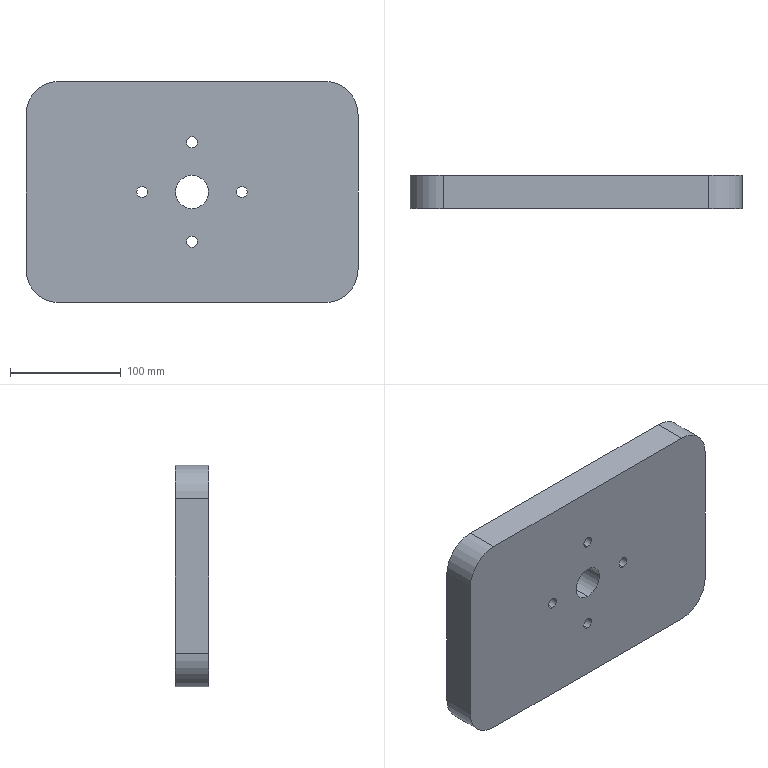Part | SolidWorks | features Extrusion 1, Fillet 1, ICE 1 | 1 solid | 20 faces | box 300 x 30 x 200 mm | volume 1746192 mm3 | cylinder 14 | plane 6 | commonest cylinder face diameters 10 x8 60 x4 30 x2
STEP:
#1=CARTESIAN_POINT('',(0.,0.,-50.));
#2=VERTEX_POINT('',#1);
#3=CARTESIAN_POINT('',(0.,0.,-40.));
#4=VERTEX_POINT('',#3);
#5=CARTESIAN_POINT('',(0.,0.,-45.));
#6=DIRECTION('',(0.,1.,0.));
#7=DIRECTION('',(0.,0.,1.));
#8=AXIS2_PLACEMENT_3D('',#5,#6,#7);
#9=CIRCLE('',#8,5.);
#10=EDGE_CURVE('',#2,#4,#9,.T.);
#11=ORIENTED_EDGE('',*,*,#10,.F.);
#12=CARTESIAN_POINT('',(0.,30.,-50.));
#13=VERTEX_POINT('',#12);
#14=CARTESIAN_POINT('',(0.,0.,-50.));
#15=DIRECTION('',(0.,1.,0.));
#16=VECTOR('',#15,1000.);
#17=LINE('',#14,#16);
#18=EDGE_CURVE('',#2,#13,#17,.T.);
#19=ORIENTED_EDGE('',*,*,#18,.T.);
#20=CARTESIAN_POINT('',(0.,30.,-40.));
#21=VERTEX_POINT('',#20);
#22=CARTESIAN_POINT('',(0.,30.,-45.));
#23=DIRECTION('',(0.,1.,0.));
#24=DIRECTION('',(0.,0.,1.));
#25=AXIS2_PLACEMENT_3D('',#22,#23,#24);
#26=CIRCLE('',#25,5.);
#27=EDGE_CURVE('',#13,#21,#26,.T.);
#28=ORIENTED_EDGE('',*,*,#27,.T.);
#29=CARTESIAN_POINT('',(0.,0.,-40.));
#30=DIRECTION('',(0.,1.,0.));
#31=VECTOR('',#30,1000.);
#32=LINE('',#29,#31);
#33=EDGE_CURVE('',#4,#21,#32,.T.);
#34=ORIENTED_EDGE('',*,*,#33,.F.);
#35=EDGE_LOOP('',(#11,#19,#28,#34));
#36=FACE_OUTER_BOUND('',#35,.T.);
#37=CARTESIAN_POINT('',(0.,0.,-45.));
#38=DIRECTION('',(0.,1.,0.));
#39=DIRECTION('',(0.,0.,1.));
#40=AXIS2_PLACEMENT_3D('',#37,#38,#39);
#41=CYLINDRICAL_SURFACE('',#40,5.);
#42=ADVANCED_FACE('',(#36),#41,.F.);
#43=CARTESIAN_POINT('',(-45.,0.,-5.));
#44=VERTEX_POINT('',#43);
#45=CARTESIAN_POINT('',(-45.,0.,5.));
#46=VERTEX_POINT('',#45);
#47=CARTESIAN_POINT('',(-45.,0.,0.));
#48=DIRECTION('',(0.,1.,0.));
#49=DIRECTION('',(0.,0.,1.));
#50=AXIS2_PLACEMENT_3D('',#47,#48,#49);
#51=CIRCLE('',#50,5.);
#52=EDGE_CURVE('',#44,#46,#51,.T.);
#53=ORIENTED_EDGE('',*,*,#52,.F.);
#54=CARTESIAN_POINT('',(-45.,30.,-5.));
#55=VERTEX_POINT('',#54);
#56=CARTESIAN_POINT('',(-45.,0.,-5.));
#57=DIRECTION('',(0.,1.,0.));
#58=VECTOR('',#57,1000.);
#59=LINE('',#56,#58);
#60=EDGE_CURVE('',#44,#55,#59,.T.);
#61=ORIENTED_EDGE('',*,*,#60,.T.);
#62=CARTESIAN_POINT('',(-45.,30.,5.));
#63=VERTEX_POINT('',#62);
#64=CARTESIAN_POINT('',(-45.,30.,0.));
#65=DIRECTION('',(0.,1.,0.));
#66=DIRECTION('',(0.,0.,1.));
#67=AXIS2_PLACEMENT_3D('',#64,#65,#66);
#68=CIRCLE('',#67,5.);
#69=EDGE_CURVE('',#55,#63,#68,.T.);
#70=ORIENTED_EDGE('',*,*,#69,.T.);
#71=CARTESIAN_POINT('',(-45.,0.,5.));
#72=DIRECTION('',(0.,1.,0.));
#73=VECTOR('',#72,1000.);
#74=LINE('',#71,#73);
#75=EDGE_CURVE('',#46,#63,#74,.T.);
#76=ORIENTED_EDGE('',*,*,#75,.F.);
#77=EDGE_LOOP('',(#53,#61,#70,#76));
#78=FACE_OUTER_BOUND('',#77,.T.);
#79=CARTESIAN_POINT('',(-45.,0.,0.));
#80=DIRECTION('',(0.,1.,0.));
#81=DIRECTION('',(0.,0.,1.));
#82=AXIS2_PLACEMENT_3D('',#79,#80,#81);
#83=CYLINDRICAL_SURFACE('',#82,5.);
#84=ADVANCED_FACE('',(#78),#83,.F.);
#85=CARTESIAN_POINT('',(0.,0.,40.));
#86=VERTEX_POINT('',#85);
#87=CARTESIAN_POINT('',(0.,0.,50.));
#88=VERTEX_POINT('',#87);
#89=CARTESIAN_POINT('',(0.,0.,45.));
#90=DIRECTION('',(0.,1.,0.));
#91=DIRECTION('',(0.,0.,-1.));
#92=AXIS2_PLACEMENT_3D('',#89,#90,#91);
#93=CIRCLE('',#92,5.);
#94=EDGE_CURVE('',#86,#88,#93,.T.);
#95=ORIENTED_EDGE('',*,*,#94,.F.);
#96=CARTESIAN_POINT('',(0.,30.,40.));
#97=VERTEX_POINT('',#96);
#98=CARTESIAN_POINT('',(0.,0.,40.));
#99=DIRECTION('',(0.,1.,0.));
#100=VECTOR('',#99,1000.);
#101=LINE('',#98,#100);
#102=EDGE_CURVE('',#86,#97,#101,.T.);
#103=ORIENTED_EDGE('',*,*,#102,.T.);
#104=CARTESIAN_POINT('',(0.,30.,50.));
#105=VERTEX_POINT('',#104);
#106=CARTESIAN_POINT('',(0.,30.,45.));
#107=DIRECTION('',(0.,1.,0.));
#108=DIRECTION('',(0.,0.,-1.));
#109=AXIS2_PLACEMENT_3D('',#106,#107,#108);
#110=CIRCLE('',#109,5.);
#111=EDGE_CURVE('',#97,#105,#110,.T.);
#112=ORIENTED_EDGE('',*,*,#111,.T.);
#113=CARTESIAN_POINT('',(0.,0.,50.));
#114=DIRECTION('',(0.,1.,0.));
#115=VECTOR('',#114,1000.);
#116=LINE('',#113,#115);
#117=EDGE_CURVE('',#88,#105,#116,.T.);
#118=ORIENTED_EDGE('',*,*,#117,.F.);
#119=EDGE_LOOP('',(#95,#103,#112,#118));
#120=FACE_OUTER_BOUND('',#119,.T.);
#121=CARTESIAN_POINT('',(0.,0.,45.));
#122=DIRECTION('',(0.,1.,0.));
#123=DIRECTION('',(0.,0.,1.));
#124=AXIS2_PLACEMENT_3D('',#121,#122,#123);
#125=CYLINDRICAL_SURFACE('',#124,5.);
#126=ADVANCED_FACE('',(#120),#125,.F.);
#127=CARTESIAN_POINT('',(45.,0.,-5.));
#128=VERTEX_POINT('',#127);
#129=CARTESIAN_POINT('',(45.,0.,5.));
#130=VERTEX_POINT('',#129);
#131=CARTESIAN_POINT('',(45.,0.,0.));
#132=DIRECTION('',(0.,1.,0.));
#133=DIRECTION('',(0.,0.,-1.));
#134=AXIS2_PLACEMENT_3D('',#131,#132,#133);
#135=CIRCLE('',#134,5.);
#136=EDGE_CURVE('',#128,#130,#135,.T.);
#137=ORIENTED_EDGE('',*,*,#136,.F.);
#138=CARTESIAN_POINT('',(45.,30.,-5.));
#139=VERTEX_POINT('',#138);
#140=CARTESIAN_POINT('',(45.,0.,-5.));
#141=DIRECTION('',(0.,1.,0.));
#142=VECTOR('',#141,1000.);
#143=LINE('',#140,#142);
#144=EDGE_CURVE('',#128,#139,#143,.T.);
#145=ORIENTED_EDGE('',*,*,#144,.T.);
#146=CARTESIAN_POINT('',(45.,30.,5.));
#147=VERTEX_POINT('',#146);
#148=CARTESIAN_POINT('',(45.,30.,0.));
#149=DIRECTION('',(0.,1.,0.));
#150=DIRECTION('',(0.,0.,-1.));
#151=AXIS2_PLACEMENT_3D('',#148,#149,#150);
#152=CIRCLE('',#151,5.);
#153=EDGE_CURVE('',#139,#147,#152,.T.);
#154=ORIENTED_EDGE('',*,*,#153,.T.);
#155=CARTESIAN_POINT('',(45.,0.,5.));
#156=DIRECTION('',(0.,1.,0.));
#157=VECTOR('',#156,1000.);
#158=LINE('',#155,#157);
#159=EDGE_CURVE('',#130,#147,#158,.T.);
#160=ORIENTED_EDGE('',*,*,#159,.F.);
#161=EDGE_LOOP('',(#137,#145,#154,#160));
#162=FACE_OUTER_BOUND('',#161,.T.);
#163=CARTESIAN_POINT('',(45.,0.,0.));
#164=DIRECTION('',(0.,1.,0.));
#165=DIRECTION('',(0.,0.,1.));
#166=AXIS2_PLACEMENT_3D('',#163,#164,#165);
#167=CYLINDRICAL_SURFACE('',#166,5.);
#168=ADVANCED_FACE('',(#162),#167,.F.);
#169=CARTESIAN_POINT('',(0.,0.,-15.));
#170=VERTEX_POINT('',#169);
#171=CARTESIAN_POINT('',(0.,0.,15.));
#172=VERTEX_POINT('',#171);
#173=CARTESIAN_POINT('',(0.,0.,0.));
#174=DIRECTION('',(0.,1.,0.));
#175=DIRECTION('',(0.,0.,1.));
#176=AXIS2_PLACEMENT_3D('',#173,#174,#175);
#177=CIRCLE('',#176,15.);
#178=EDGE_CURVE('',#170,#172,#177,.T.);
#179=ORIENTED_EDGE('',*,*,#178,.F.);
#180=CARTESIAN_POINT('',(0.,30.,-15.));
#181=VERTEX_POINT('',#180);
#182=CARTESIAN_POINT('',(0.,0.,-15.));
#183=DIRECTION('',(0.,1.,0.));
#184=VECTOR('',#183,1000.);
#185=LINE('',#182,#184);
#186=EDGE_CURVE('',#170,#181,#185,.T.);
#187=ORIENTED_EDGE('',*,*,#186,.T.);
#188=CARTESIAN_POINT('',(0.,30.,15.));
#189=VERTEX_POINT('',#188);
#190=CARTESIAN_POINT('',(0.,30.,0.));
#191=DIRECTION('',(0.,1.,0.));
#192=DIRECTION('',(0.,0.,1.));
#193=AXIS2_PLACEMENT_3D('',#190,#191,#192);
#194=CIRCLE('',#193,15.);
#195=EDGE_CURVE('',#181,#189,#194,.T.);
#196=ORIENTED_EDGE('',*,*,#195,.T.);
#197=CARTESIAN_POINT('',(0.,0.,15.));
#198=DIRECTION('',(0.,1.,0.));
#199=VECTOR('',#198,1000.);
#200=LINE('',#197,#199);
#201=EDGE_CURVE('',#172,#189,#200,.T.);
#202=ORIENTED_EDGE('',*,*,#201,.F.);
#203=EDGE_LOOP('',(#179,#187,#196,#202));
#204=FACE_OUTER_BOUND('',#203,.T.);
#205=CARTESIAN_POINT('',(0.,0.,0.));
#206=DIRECTION('',(0.,1.,0.));
#207=DIRECTION('',(0.,0.,1.));
#208=AXIS2_PLACEMENT_3D('',#205,#206,#207);
#209=CYLINDRICAL_SURFACE('',#208,15.);
#210=ADVANCED_FACE('',(#204),#209,.F.);
#211=CARTESIAN_POINT('',(150.,0.,70.));
#212=VERTEX_POINT('',#211);
#213=CARTESIAN_POINT('',(150.,0.,-70.));
#214=VERTEX_POINT('',#213);
#215=CARTESIAN_POINT('',(150.,0.,100.));
#216=DIRECTION('',(0.,0.,-1.));
#217=VECTOR('',#216,1000.);
#218=LINE('',#215,#217);
#219=EDGE_CURVE('',#212,#214,#218,.T.);
#220=ORIENTED_EDGE('',*,*,#219,.T.);
#221=CARTESIAN_POINT('',(150.,30.,-70.));
#222=VERTEX_POINT('',#221);
#223=CARTESIAN_POINT('',(150.,30.,-70.));
#224=DIRECTION('',(0.,1.,0.));
#225=VECTOR('',#224,1000.);
#226=LINE('',#223,#225);
#227=EDGE_CURVE('',#214,#222,#226,.T.);
#228=ORIENTED_EDGE('',*,*,#227,.T.);
#229=CARTESIAN_POINT('',(150.,30.,70.));
#230=VERTEX_POINT('',#229);
#231=CARTESIAN_POINT('',(150.,30.,100.));
#232=DIRECTION('',(0.,0.,-1.));
#233=VECTOR('',#232,1000.);
#234=LINE('',#231,#233);
#235=EDGE_CURVE('',#230,#222,#234,.T.);
#236=ORIENTED_EDGE('',*,*,#235,.F.);
#237=CARTESIAN_POINT('',(150.,30.,70.));
#238=DIRECTION('',(0.,-1.,0.));
#239=VECTOR('',#238,1000.);
#240=LINE('',#237,#239);
#241=EDGE_CURVE('',#230,#212,#240,.T.);
#242=ORIENTED_EDGE('',*,*,#241,.T.);
#243=EDGE_LOOP('',(#220,#228,#236,#242));
#244=FACE_OUTER_BOUND('',#243,.T.);
#245=CARTESIAN_POINT('',(150.,30.,100.));
#246=DIRECTION('',(-1.,0.,0.));
#247=DIRECTION('',(0.,0.,1.));
#248=AXIS2_PLACEMENT_3D('',#245,#246,#247);
#249=PLANE('',#248);
#250=ADVANCED_FACE('',(#244),#249,.F.);
#251=CARTESIAN_POINT('',(120.,0.,-100.));
#252=VERTEX_POINT('',#251);
#253=CARTESIAN_POINT('',(-120.,0.,-100.));
#254=VERTEX_POINT('',#253);
#255=CARTESIAN_POINT('',(-150.,0.,-100.));
#256=DIRECTION('',(-1.,0.,0.));
#257=VECTOR('',#256,1000.);
#258=LINE('',#255,#257);
#259=EDGE_CURVE('',#252,#254,#258,.T.);
#260=ORIENTED_EDGE('',*,*,#259,.T.);
#261=CARTESIAN_POINT('',(-120.,30.,-100.));
#262=VERTEX_POINT('',#261);
#263=CARTESIAN_POINT('',(-120.,30.,-100.));
#264=DIRECTION('',(0.,1.,0.));
#265=VECTOR('',#264,1000.);
#266=LINE('',#263,#265);
#267=EDGE_CURVE('',#254,#262,#266,.T.);
#268=ORIENTED_EDGE('',*,*,#267,.T.);
#269=CARTESIAN_POINT('',(120.,30.,-100.));
#270=VERTEX_POINT('',#269);
#271=CARTESIAN_POINT('',(-150.,30.,-100.));
#272=DIRECTION('',(-1.,0.,0.));
#273=VECTOR('',#272,1000.);
#274=LINE('',#271,#273);
#275=EDGE_CURVE('',#270,#262,#274,.T.);
#276=ORIENTED_EDGE('',*,*,#275,.F.);
#277=CARTESIAN_POINT('',(120.,30.,-100.));
#278=DIRECTION('',(0.,-1.,0.));
#279=VECTOR('',#278,1000.);
#280=LINE('',#277,#279);
#281=EDGE_CURVE('',#270,#252,#280,.T.);
#282=ORIENTED_EDGE('',*,*,#281,.T.);
#283=EDGE_LOOP('',(#260,#268,#276,#282));
#284=FACE_OUTER_BOUND('',#283,.T.);
#285=CARTESIAN_POINT('',(-150.,30.,-100.));
#286=DIRECTION('',(0.,0.,1.));
#287=DIRECTION('',(1.,0.,0.));
#288=AXIS2_PLACEMENT_3D('',#285,#286,#287);
#289=PLANE('',#288);
#290=ADVANCED_FACE('',(#284),#289,.F.);
#291=CARTESIAN_POINT('',(-150.,0.,-70.));
#292=VERTEX_POINT('',#291);
#293=CARTESIAN_POINT('',(-150.,0.,70.));
#294=VERTEX_POINT('',#293);
#295=CARTESIAN_POINT('',(-150.,0.,100.));
#296=DIRECTION('',(0.,0.,1.));
#297=VECTOR('',#296,1000.);
#298=LINE('',#295,#297);
#299=EDGE_CURVE('',#292,#294,#298,.T.);
#300=ORIENTED_EDGE('',*,*,#299,.T.);
#301=CARTESIAN_POINT('',(-150.,30.,70.));
#302=VERTEX_POINT('',#301);
#303=CARTESIAN_POINT('',(-150.,30.,70.));
#304=DIRECTION('',(0.,1.,0.));
#305=VECTOR('',#304,1000.);
#306=LINE('',#303,#305);
#307=EDGE_CURVE('',#294,#302,#306,.T.);
#308=ORIENTED_EDGE('',*,*,#307,.T.);
#309=CARTESIAN_POINT('',(-150.,30.,-70.));
#310=VERTEX_POINT('',#309);
#311=CARTESIAN_POINT('',(-150.,30.,100.));
#312=DIRECTION('',(0.,0.,1.));
#313=VECTOR('',#312,1000.);
#314=LINE('',#311,#313);
#315=EDGE_CURVE('',#310,#302,#314,.T.);
#316=ORIENTED_EDGE('',*,*,#315,.F.);
#317=CARTESIAN_POINT('',(-150.,30.,-70.));
#318=DIRECTION('',(0.,-1.,0.));
#319=VECTOR('',#318,1000.);
#320=LINE('',#317,#319);
#321=EDGE_CURVE('',#310,#292,#320,.T.);
#322=ORIENTED_EDGE('',*,*,#321,.T.);
#323=EDGE_LOOP('',(#300,#308,#316,#322));
#324=FACE_OUTER_BOUND('',#323,.T.);
#325=CARTESIAN_POINT('',(-150.,30.,100.));
#326=DIRECTION('',(1.,0.,0.));
#327=DIRECTION('',(0.,0.,-1.));
#328=AXIS2_PLACEMENT_3D('',#325,#326,#327);
#329=PLANE('',#328);
#330=ADVANCED_FACE('',(#324),#329,.F.);
#331=CARTESIAN_POINT('',(-120.,30.,100.));
#332=VERTEX_POINT('',#331);
#333=CARTESIAN_POINT('',(120.,30.,100.));
#334=VERTEX_POINT('',#333);
#335=CARTESIAN_POINT('',(-150.,30.,100.));
#336=DIRECTION('',(1.,0.,0.));
#337=VECTOR('',#336,1000.);
#338=LINE('',#335,#337);
#339=EDGE_CURVE('',#332,#334,#338,.T.);
#340=ORIENTED_EDGE('',*,*,#339,.F.);
#341=CARTESIAN_POINT('',(-120.,0.,100.));
#342=VERTEX_POINT('',#341);
#343=CARTESIAN_POINT('',(-120.,30.,100.));
#344=DIRECTION('',(0.,-1.,0.));
#345=VECTOR('',#344,1000.);
#346=LINE('',#343,#345);
#347=EDGE_CURVE('',#332,#342,#346,.T.);
#348=ORIENTED_EDGE('',*,*,#347,.T.);
#349=CARTESIAN_POINT('',(120.,0.,100.));
#350=VERTEX_POINT('',#349);
#351=CARTESIAN_POINT('',(-150.,0.,100.));
#352=DIRECTION('',(1.,0.,0.));
#353=VECTOR('',#352,1000.);
#354=LINE('',#351,#353);
#355=EDGE_CURVE('',#342,#350,#354,.T.);
#356=ORIENTED_EDGE('',*,*,#355,.T.);
#357=CARTESIAN_POINT('',(120.,30.,100.));
#358=DIRECTION('',(0.,1.,0.));
#359=VECTOR('',#358,1000.);
#360=LINE('',#357,#359);
#361=EDGE_CURVE('',#350,#334,#360,.T.);
#362=ORIENTED_EDGE('',*,*,#361,.T.);
#363=EDGE_LOOP('',(#340,#348,#356,#362));
#364=FACE_OUTER_BOUND('',#363,.T.);
#365=CARTESIAN_POINT('',(-150.,30.,100.));
#366=DIRECTION('',(0.,0.,-1.));
#367=DIRECTION('',(-1.,0.,0.));
#368=AXIS2_PLACEMENT_3D('',#365,#366,#367);
#369=PLANE('',#368);
#370=ADVANCED_FACE('',(#364),#369,.F.);
#371=CARTESIAN_POINT('',(0.,30.,-45.));
#372=DIRECTION('',(0.,1.,0.));
#373=DIRECTION('',(0.,0.,1.));
#374=AXIS2_PLACEMENT_3D('',#371,#372,#373);
#375=CIRCLE('',#374,5.);
#376=EDGE_CURVE('',#21,#13,#375,.T.);
#377=ORIENTED_EDGE('',*,*,#376,.F.);
#378=ORIENTED_EDGE('',*,*,#27,.F.);
#379=EDGE_LOOP('',(#377,#378));
#380=FACE_BOUND('',#379,.T.);
#381=CARTESIAN_POINT('',(-45.,30.,0.));
#382=DIRECTION('',(0.,1.,0.));
#383=DIRECTION('',(0.,0.,1.));
#384=AXIS2_PLACEMENT_3D('',#381,#382,#383);
#385=CIRCLE('',#384,5.);
#386=EDGE_CURVE('',#63,#55,#385,.T.);
#387=ORIENTED_EDGE('',*,*,#386,.F.);
#388=ORIENTED_EDGE('',*,*,#69,.F.);
#389=EDGE_LOOP('',(#387,#388));
#390=FACE_BOUND('',#389,.T.);
#391=CARTESIAN_POINT('',(0.,30.,45.));
#392=DIRECTION('',(0.,1.,0.));
#393=DIRECTION('',(0.,0.,-1.));
#394=AXIS2_PLACEMENT_3D('',#391,#392,#393);
#395=CIRCLE('',#394,5.);
#396=EDGE_CURVE('',#105,#97,#395,.T.);
#397=ORIENTED_EDGE('',*,*,#396,.F.);
#398=ORIENTED_EDGE('',*,*,#111,.F.);
#399=EDGE_LOOP('',(#397,#398));
#400=FACE_BOUND('',#399,.T.);
#401=CARTESIAN_POINT('',(45.,30.,0.));
#402=DIRECTION('',(0.,1.,0.));
#403=DIRECTION('',(0.,0.,-1.));
#404=AXIS2_PLACEMENT_3D('',#401,#402,#403);
#405=CIRCLE('',#404,5.);
#406=EDGE_CURVE('',#147,#139,#405,.T.);
#407=ORIENTED_EDGE('',*,*,#406,.F.);
#408=ORIENTED_EDGE('',*,*,#153,.F.);
#409=EDGE_LOOP('',(#407,#408));
#410=FACE_BOUND('',#409,.T.);
#411=CARTESIAN_POINT('',(0.,30.,0.));
#412=DIRECTION('',(0.,1.,0.));
#413=DIRECTION('',(0.,0.,1.));
#414=AXIS2_PLACEMENT_3D('',#411,#412,#413);
#415=CIRCLE('',#414,15.);
#416=EDGE_CURVE('',#189,#181,#415,.T.);
#417=ORIENTED_EDGE('',*,*,#416,.F.);
#418=ORIENTED_EDGE('',*,*,#195,.F.);
#419=EDGE_LOOP('',(#417,#418));
#420=FACE_BOUND('',#419,.T.);
#421=ORIENTED_EDGE('',*,*,#315,.T.);
#422=CARTESIAN_POINT('',(-120.,30.,70.));
#423=DIRECTION('',(0.,1.,0.));
#424=DIRECTION('',(0.,0.,-1.));
#425=AXIS2_PLACEMENT_3D('',#422,#423,#424);
#426=CIRCLE('',#425,30.);
#427=EDGE_CURVE('',#302,#332,#426,.T.);
#428=ORIENTED_EDGE('',*,*,#427,.T.);
#429=ORIENTED_EDGE('',*,*,#339,.T.);
#430=CARTESIAN_POINT('',(120.,30.,70.));
#431=DIRECTION('',(0.,1.,0.));
#432=DIRECTION('',(0.,0.,-1.));
#433=AXIS2_PLACEMENT_3D('',#430,#431,#432);
#434=CIRCLE('',#433,30.);
#435=EDGE_CURVE('',#334,#230,#434,.T.);
#436=ORIENTED_EDGE('',*,*,#435,.T.);
#437=ORIENTED_EDGE('',*,*,#235,.T.);
#438=CARTESIAN_POINT('',(120.,30.,-70.));
#439=DIRECTION('',(0.,1.,0.));
#440=DIRECTION('',(0.,0.,-1.));
#441=AXIS2_PLACEMENT_3D('',#438,#439,#440);
#442=CIRCLE('',#441,30.);
#443=EDGE_CURVE('',#222,#270,#442,.T.);
#444=ORIENTED_EDGE('',*,*,#443,.T.);
#445=ORIENTED_EDGE('',*,*,#275,.T.);
#446=CARTESIAN_POINT('',(-120.,30.,-70.));
#447=DIRECTION('',(0.,1.,0.));
#448=DIRECTION('',(0.,0.,-1.));
#449=AXIS2_PLACEMENT_3D('',#446,#447,#448);
#450=CIRCLE('',#449,30.);
#451=EDGE_CURVE('',#262,#310,#450,.T.);
#452=ORIENTED_EDGE('',*,*,#451,.T.);
#453=EDGE_LOOP('',(#421,#428,#429,#436,#437,#444,#445,#452));
#454=FACE_OUTER_BOUND('',#453,.T.);
#455=CARTESIAN_POINT('',(0.,30.,0.));
#456=DIRECTION('',(0.,-1.,0.));
#457=DIRECTION('',(0.,0.,-1.));
#458=AXIS2_PLACEMENT_3D('',#455,#456,#457);
#459=PLANE('',#458);
#460=ADVANCED_FACE('',(#380,#390,#400,#410,#420,#454),#459,.F.);
#461=CARTESIAN_POINT('',(0.,0.,-45.));
#462=DIRECTION('',(0.,1.,0.));
#463=DIRECTION('',(0.,0.,1.));
#464=AXIS2_PLACEMENT_3D('',#461,#462,#463);
#465=CIRCLE('',#464,5.);
#466=EDGE_CURVE('',#4,#2,#465,.T.);
#467=ORIENTED_EDGE('',*,*,#466,.T.);
#468=ORIENTED_EDGE('',*,*,#10,.T.);
#469=EDGE_LOOP('',(#467,#468));
#470=FACE_BOUND('',#469,.T.);
#471=CARTESIAN_POINT('',(-45.,0.,0.));
#472=DIRECTION('',(0.,1.,0.));
#473=DIRECTION('',(0.,0.,1.));
#474=AXIS2_PLACEMENT_3D('',#471,#472,#473);
#475=CIRCLE('',#474,5.);
#476=EDGE_CURVE('',#46,#44,#475,.T.);
#477=ORIENTED_EDGE('',*,*,#476,.T.);
#478=ORIENTED_EDGE('',*,*,#52,.T.);
#479=EDGE_LOOP('',(#477,#478));
#480=FACE_BOUND('',#479,.T.);
#481=CARTESIAN_POINT('',(0.,0.,45.));
#482=DIRECTION('',(0.,1.,0.));
#483=DIRECTION('',(0.,0.,-1.));
#484=AXIS2_PLACEMENT_3D('',#481,#482,#483);
#485=CIRCLE('',#484,5.);
#486=EDGE_CURVE('',#88,#86,#485,.T.);
#487=ORIENTED_EDGE('',*,*,#486,.T.);
#488=ORIENTED_EDGE('',*,*,#94,.T.);
#489=EDGE_LOOP('',(#487,#488));
#490=FACE_BOUND('',#489,.T.);
#491=CARTESIAN_POINT('',(45.,0.,0.));
#492=DIRECTION('',(0.,1.,0.));
#493=DIRECTION('',(0.,0.,-1.));
#494=AXIS2_PLACEMENT_3D('',#491,#492,#493);
#495=CIRCLE('',#494,5.);
#496=EDGE_CURVE('',#130,#128,#495,.T.);
#497=ORIENTED_EDGE('',*,*,#496,.T.);
#498=ORIENTED_EDGE('',*,*,#136,.T.);
#499=EDGE_LOOP('',(#497,#498));
#500=FACE_BOUND('',#499,.T.);
#501=CARTESIAN_POINT('',(0.,0.,0.));
#502=DIRECTION('',(0.,1.,0.));
#503=DIRECTION('',(0.,0.,1.));
#504=AXIS2_PLACEMENT_3D('',#501,#502,#503);
#505=CIRCLE('',#504,15.);
#506=EDGE_CURVE('',#172,#170,#505,.T.);
#507=ORIENTED_EDGE('',*,*,#506,.T.);
#508=ORIENTED_EDGE('',*,*,#178,.T.);
#509=EDGE_LOOP('',(#507,#508));
#510=FACE_BOUND('',#509,.T.);
#511=ORIENTED_EDGE('',*,*,#355,.F.);
#512=CARTESIAN_POINT('',(-120.,0.,70.));
#513=DIRECTION('',(0.,-1.,0.));
#514=DIRECTION('',(0.,0.,-1.));
#515=AXIS2_PLACEMENT_3D('',#512,#513,#514);
#516=CIRCLE('',#515,30.);
#517=EDGE_CURVE('',#342,#294,#516,.T.);
#518=ORIENTED_EDGE('',*,*,#517,.T.);
#519=ORIENTED_EDGE('',*,*,#299,.F.);
#520=CARTESIAN_POINT('',(-120.,0.,-70.));
#521=DIRECTION('',(0.,-1.,0.));
#522=DIRECTION('',(0.,0.,-1.));
#523=AXIS2_PLACEMENT_3D('',#520,#521,#522);
#524=CIRCLE('',#523,30.);
#525=EDGE_CURVE('',#292,#254,#524,.T.);
#526=ORIENTED_EDGE('',*,*,#525,.T.);
#527=ORIENTED_EDGE('',*,*,#259,.F.);
#528=CARTESIAN_POINT('',(120.,0.,-70.));
#529=DIRECTION('',(0.,-1.,0.));
#530=DIRECTION('',(0.,0.,-1.));
#531=AXIS2_PLACEMENT_3D('',#528,#529,#530);
#532=CIRCLE('',#531,30.);
#533=EDGE_CURVE('',#252,#214,#532,.T.);
#534=ORIENTED_EDGE('',*,*,#533,.T.);
#535=ORIENTED_EDGE('',*,*,#219,.F.);
#536=CARTESIAN_POINT('',(120.,0.,70.));
#537=DIRECTION('',(0.,-1.,0.));
#538=DIRECTION('',(0.,0.,-1.));
#539=AXIS2_PLACEMENT_3D('',#536,#537,#538);
#540=CIRCLE('',#539,30.);
#541=EDGE_CURVE('',#212,#350,#540,.T.);
#542=ORIENTED_EDGE('',*,*,#541,.T.);
#543=EDGE_LOOP('',(#511,#518,#519,#526,#527,#534,#535,#542));
#544=FACE_OUTER_BOUND('',#543,.T.);
#545=CARTESIAN_POINT('',(0.,0.,0.));
#546=DIRECTION('',(0.,-1.,0.));
#547=DIRECTION('',(0.,0.,-1.));
#548=AXIS2_PLACEMENT_3D('',#545,#546,#547);
#549=PLANE('',#548);
#550=ADVANCED_FACE('',(#470,#480,#490,#500,#510,#544),#549,.T.);
#551=ORIENTED_EDGE('',*,*,#186,.F.);
#552=ORIENTED_EDGE('',*,*,#506,.F.);
#553=ORIENTED_EDGE('',*,*,#201,.T.);
#554=ORIENTED_EDGE('',*,*,#416,.T.);
#555=EDGE_LOOP('',(#551,#552,#553,#554));
#556=FACE_OUTER_BOUND('',#555,.T.);
#557=CARTESIAN_POINT('',(0.,0.,0.));
#558=DIRECTION('',(0.,1.,0.));
#559=DIRECTION('',(0.,0.,1.));
#560=AXIS2_PLACEMENT_3D('',#557,#558,#559);
#561=CYLINDRICAL_SURFACE('',#560,15.);
#562=ADVANCED_FACE('',(#556),#561,.F.);
#563=ORIENTED_EDGE('',*,*,#144,.F.);
#564=ORIENTED_EDGE('',*,*,#496,.F.);
#565=ORIENTED_EDGE('',*,*,#159,.T.);
#566=ORIENTED_EDGE('',*,*,#406,.T.);
#567=EDGE_LOOP('',(#563,#564,#565,#566));
#568=FACE_OUTER_BOUND('',#567,.T.);
#569=CARTESIAN_POINT('',(45.,0.,0.));
#570=DIRECTION('',(0.,1.,0.));
#571=DIRECTION('',(0.,0.,1.));
#572=AXIS2_PLACEMENT_3D('',#569,#570,#571);
#573=CYLINDRICAL_SURFACE('',#572,5.);
#574=ADVANCED_FACE('',(#568),#573,.F.);
#575=ORIENTED_EDGE('',*,*,#102,.F.);
#576=ORIENTED_EDGE('',*,*,#486,.F.);
#577=ORIENTED_EDGE('',*,*,#117,.T.);
#578=ORIENTED_EDGE('',*,*,#396,.T.);
#579=EDGE_LOOP('',(#575,#576,#577,#578));
#580=FACE_OUTER_BOUND('',#579,.T.);
#581=CARTESIAN_POINT('',(0.,0.,45.));
#582=DIRECTION('',(0.,1.,0.));
#583=DIRECTION('',(0.,0.,1.));
#584=AXIS2_PLACEMENT_3D('',#581,#582,#583);
#585=CYLINDRICAL_SURFACE('',#584,5.);
#586=ADVANCED_FACE('',(#580),#585,.F.);
#587=ORIENTED_EDGE('',*,*,#60,.F.);
#588=ORIENTED_EDGE('',*,*,#476,.F.);
#589=ORIENTED_EDGE('',*,*,#75,.T.);
#590=ORIENTED_EDGE('',*,*,#386,.T.);
#591=EDGE_LOOP('',(#587,#588,#589,#590));
#592=FACE_OUTER_BOUND('',#591,.T.);
#593=CARTESIAN_POINT('',(-45.,0.,0.));
#594=DIRECTION('',(0.,1.,0.));
#595=DIRECTION('',(0.,0.,1.));
#596=AXIS2_PLACEMENT_3D('',#593,#594,#595);
#597=CYLINDRICAL_SURFACE('',#596,5.);
#598=ADVANCED_FACE('',(#592),#597,.F.);
#599=ORIENTED_EDGE('',*,*,#18,.F.);
#600=ORIENTED_EDGE('',*,*,#466,.F.);
#601=ORIENTED_EDGE('',*,*,#33,.T.);
#602=ORIENTED_EDGE('',*,*,#376,.T.);
#603=EDGE_LOOP('',(#599,#600,#601,#602));
#604=FACE_OUTER_BOUND('',#603,.T.);
#605=CARTESIAN_POINT('',(0.,0.,-45.));
#606=DIRECTION('',(0.,1.,0.));
#607=DIRECTION('',(0.,0.,1.));
#608=AXIS2_PLACEMENT_3D('',#605,#606,#607);
#609=CYLINDRICAL_SURFACE('',#608,5.);
#610=ADVANCED_FACE('',(#604),#609,.F.);
#611=ORIENTED_EDGE('',*,*,#427,.F.);
#612=ORIENTED_EDGE('',*,*,#307,.F.);
#613=ORIENTED_EDGE('',*,*,#517,.F.);
#614=ORIENTED_EDGE('',*,*,#347,.F.);
#615=EDGE_LOOP('',(#611,#612,#613,#614));
#616=FACE_OUTER_BOUND('',#615,.T.);
#617=CARTESIAN_POINT('',(-120.,30.,70.));
#618=DIRECTION('',(0.,-1.,0.));
#619=DIRECTION('',(0.,0.,-1.));
#620=AXIS2_PLACEMENT_3D('',#617,#618,#619);
#621=CYLINDRICAL_SURFACE('',#620,30.);
#622=ADVANCED_FACE('',(#616),#621,.T.);
#623=ORIENTED_EDGE('',*,*,#451,.F.);
#624=ORIENTED_EDGE('',*,*,#267,.F.);
#625=ORIENTED_EDGE('',*,*,#525,.F.);
#626=ORIENTED_EDGE('',*,*,#321,.F.);
#627=EDGE_LOOP('',(#623,#624,#625,#626));
#628=FACE_OUTER_BOUND('',#627,.T.);
#629=CARTESIAN_POINT('',(-120.,30.,-70.));
#630=DIRECTION('',(0.,-1.,0.));
#631=DIRECTION('',(0.,0.,-1.));
#632=AXIS2_PLACEMENT_3D('',#629,#630,#631);
#633=CYLINDRICAL_SURFACE('',#632,30.);
#634=ADVANCED_FACE('',(#628),#633,.T.);
#635=ORIENTED_EDGE('',*,*,#443,.F.);
#636=ORIENTED_EDGE('',*,*,#227,.F.);
#637=ORIENTED_EDGE('',*,*,#533,.F.);
#638=ORIENTED_EDGE('',*,*,#281,.F.);
#639=EDGE_LOOP('',(#635,#636,#637,#638));
#640=FACE_OUTER_BOUND('',#639,.T.);
#641=CARTESIAN_POINT('',(120.,30.,-70.));
#642=DIRECTION('',(0.,-1.,0.));
#643=DIRECTION('',(0.,0.,-1.));
#644=AXIS2_PLACEMENT_3D('',#641,#642,#643);
#645=CYLINDRICAL_SURFACE('',#644,30.);
#646=ADVANCED_FACE('',(#640),#645,.T.);
#647=ORIENTED_EDGE('',*,*,#435,.F.);
#648=ORIENTED_EDGE('',*,*,#361,.F.);
#649=ORIENTED_EDGE('',*,*,#541,.F.);
#650=ORIENTED_EDGE('',*,*,#241,.F.);
#651=EDGE_LOOP('',(#647,#648,#649,#650));
#652=FACE_OUTER_BOUND('',#651,.T.);
#653=CARTESIAN_POINT('',(120.,30.,70.));
#654=DIRECTION('',(0.,-1.,0.));
#655=DIRECTION('',(0.,0.,-1.));
#656=AXIS2_PLACEMENT_3D('',#653,#654,#655);
#657=CYLINDRICAL_SURFACE('',#656,30.);
#658=ADVANCED_FACE('',(#652),#657,.T.);
#659=CLOSED_SHELL('',(#42,#84,#126,#168,#210,#250,#290,#330,#370,#460,#550,#562,#574,#586,#598,#610,#622,#634,#646,#658));
#660=MANIFOLD_SOLID_BREP('',#659);
#661=CARTESIAN_POINT('',(0.,0.,0.));
#662=DIRECTION('',(0.,0.,1.));
#663=DIRECTION('',(1.,0.,0.));
#664=AXIS2_PLACEMENT_3D('',#661,#662,#663);
#665=(LENGTH_UNIT()NAMED_UNIT(*)SI_UNIT(.MILLI.,.METRE.));
#666=UNCERTAINTY_MEASURE_WITH_UNIT(LENGTH_MEASURE(0.00001),#665,'','');
#667=(NAMED_UNIT(*)PLANE_ANGLE_UNIT()SI_UNIT($,.RADIAN.));
#668=(NAMED_UNIT(*)SI_UNIT($,.STERADIAN.)SOLID_ANGLE_UNIT());
#669=(GEOMETRIC_REPRESENTATION_CONTEXT(3)GLOBAL_UNCERTAINTY_ASSIGNED_CONTEXT((#666))GLOBAL_UNIT_ASSIGNED_CONTEXT((#665,#667,#668))REPRESENTATION_CONTEXT('',''));
#670=ADVANCED_BREP_SHAPE_REPRESENTATION('',(#660,#664),#669);